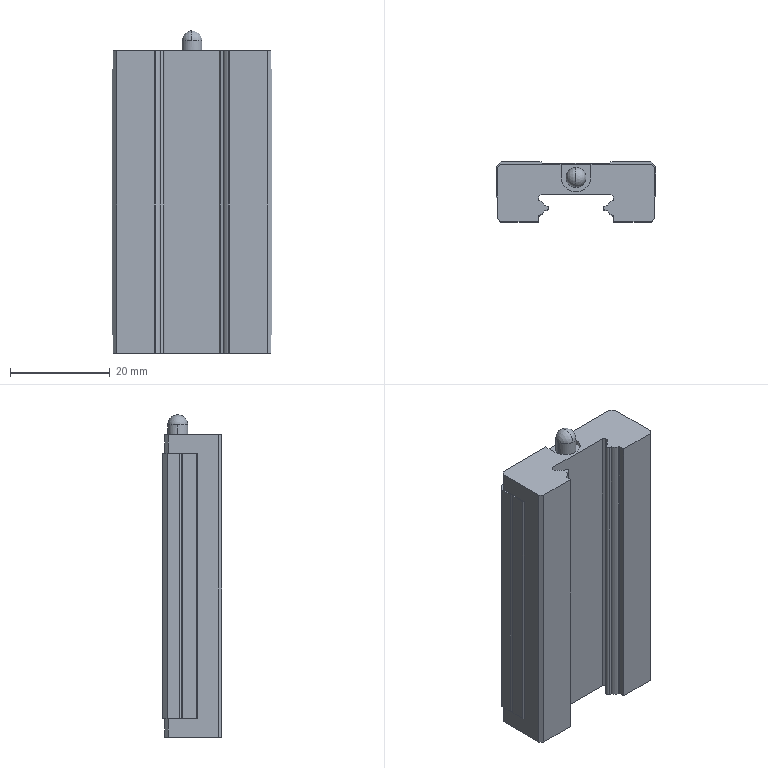Part | NX | features BREP 1 | 1 solid | 88 faces | box 32 x 12 x 64.5 mm | volume 18041 mm3 | plane 45 | cylinder 25 | cone 16 | sphere 2 | commonest cylinder face diameters 2.459 x8 0.4 x4 3.43 x4 0.8 x3 1 x2 4 x2